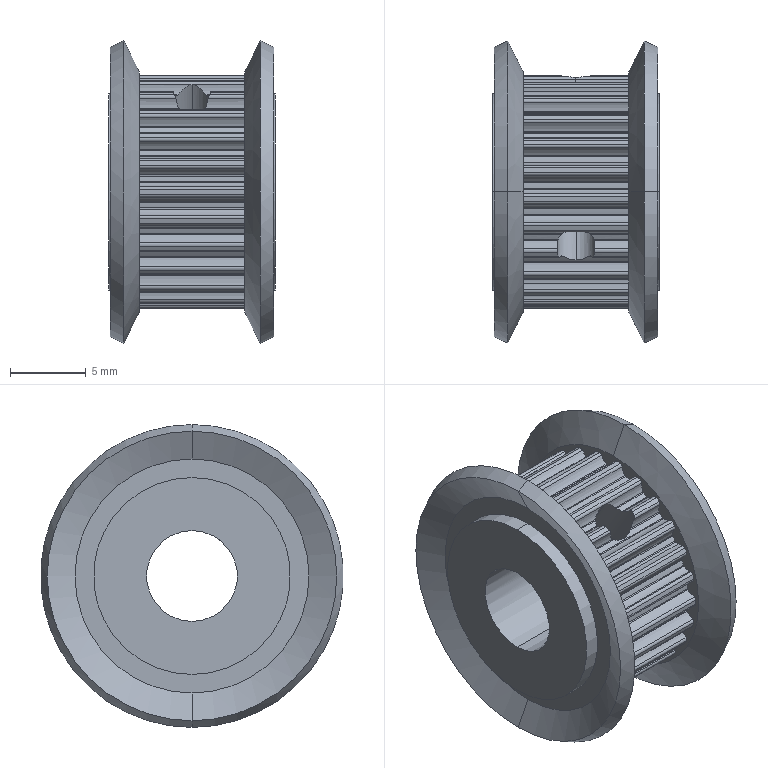Part | SolidWorks | features BaseBody 1, CirPattern 1, HoleWzd 1, ICE 1 | 1 solid | 269 faces | box 11 x 20 x 20 mm | volume 1710 mm3 | cylinder 251 | cone 12 | plane 6 | commonest cylinder face diameters 0.38 x65 0.2 x62 2.65 x59 15.41 x28 13.89 x27 2.5 x4